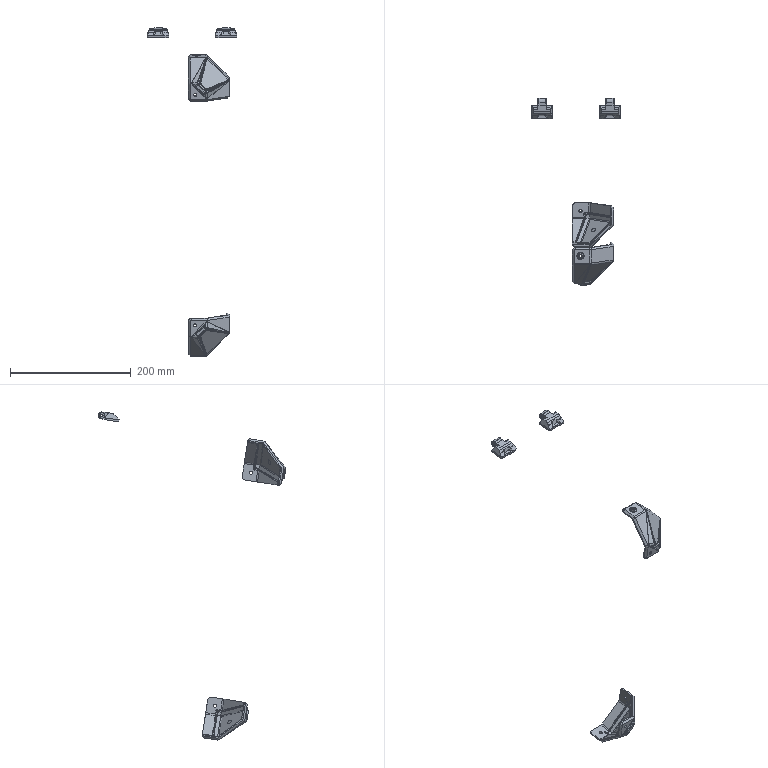Part | SolidWorks | features BaseBody 4 | 4 solids | 846 faces | box 147.369 x 309.684 x 542.282 mm | volume 88870 mm3 | cylinder 390 | plane 204 | spline 154 | cone 50 | sphere 32 | torus 16 | commonest cylinder face diameters 3 x72 5 x72 4.4 x62 8 x34 10 x28 2 x20